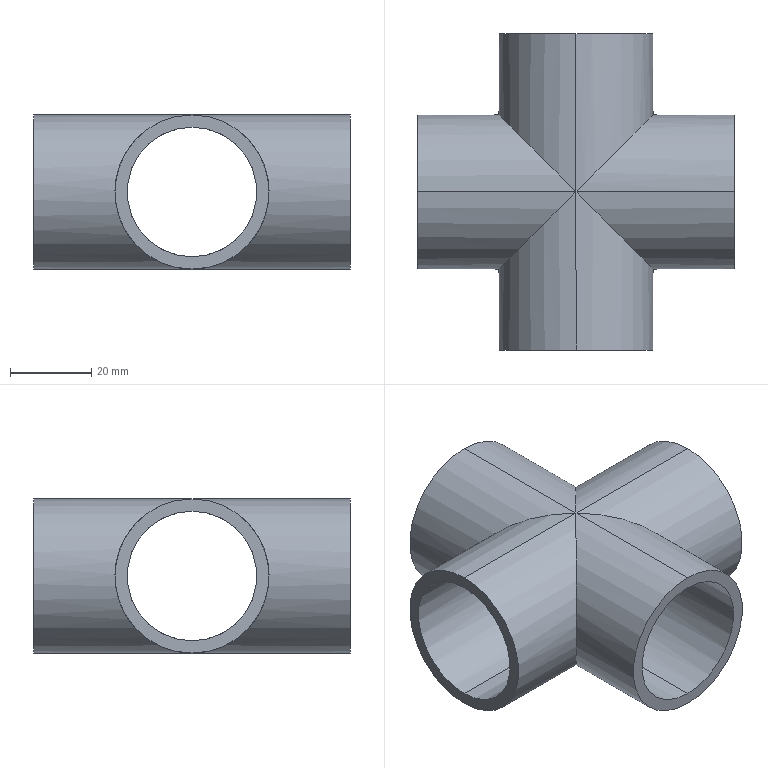Part | SolidWorks | features ICE 2, CirPattern 1, RefAxis 1, Revolution 1 | 1 solid | 20 faces | box 78 x 78 x 38 mm | volume 36723 mm3 | cylinder 16 | plane 4 | commonest cylinder face diameters 32 x8 38 x8
STEP:
#1=CARTESIAN_POINT('',(-39.,0.,16.));
#2=VERTEX_POINT('',#1);
#3=CARTESIAN_POINT('',(-39.,0.,-16.));
#4=VERTEX_POINT('',#3);
#5=CARTESIAN_POINT('',(-39.,0.,0.));
#6=DIRECTION('',(1.,0.,0.));
#7=DIRECTION('',(0.,0.,-1.));
#8=AXIS2_PLACEMENT_3D('',#5,#6,#7);
#9=CIRCLE('',#8,16.);
#10=EDGE_CURVE('',#2,#4,#9,.T.);
#11=ORIENTED_EDGE('',*,*,#10,.F.);
#12=CARTESIAN_POINT('',(0.,0.,16.));
#13=VERTEX_POINT('',#12);
#14=CARTESIAN_POINT('',(0.,0.,16.));
#15=DIRECTION('',(1.,0.,0.));
#16=VECTOR('',#15,1000.);
#17=LINE('',#14,#16);
#18=EDGE_CURVE('',#2,#13,#17,.T.);
#19=ORIENTED_EDGE('',*,*,#18,.T.);
#20=CARTESIAN_POINT('',(0.,0.,-16.));
#21=VERTEX_POINT('',#20);
#22=CARTESIAN_POINT('',(0.,0.,-16.));
#23=CARTESIAN_POINT('',(-32.,-32.,-16.));
#24=CARTESIAN_POINT('',(-32.,-32.,16.));
#25=CARTESIAN_POINT('',(0.,0.,16.));
#26=(BOUNDED_CURVE()B_SPLINE_CURVE(3,(#22,#23,#24,#25),.UNSPECIFIED.,.F.,.T.)B_SPLINE_CURVE_WITH_KNOTS((4,4),(4.712,7.854),.UNSPECIFIED.)CURVE()GEOMETRIC_REPRESENTATION_ITEM()RATIONAL_B_SPLINE_CURVE((1.,0.3333,0.3333,1.))REPRESENTATION_ITEM(''));
#27=EDGE_CURVE('',#21,#13,#26,.T.);
#28=ORIENTED_EDGE('',*,*,#27,.F.);
#29=CARTESIAN_POINT('',(0.,0.,-16.));
#30=DIRECTION('',(1.,0.,0.));
#31=VECTOR('',#30,1000.);
#32=LINE('',#29,#31);
#33=EDGE_CURVE('',#4,#21,#32,.T.);
#34=ORIENTED_EDGE('',*,*,#33,.F.);
#35=EDGE_LOOP('',(#11,#19,#28,#34));
#36=FACE_OUTER_BOUND('',#35,.T.);
#37=CARTESIAN_POINT('',(0.,0.,0.));
#38=DIRECTION('',(1.,0.,0.));
#39=DIRECTION('',(0.,0.,-1.));
#40=AXIS2_PLACEMENT_3D('',#37,#38,#39);
#41=CYLINDRICAL_SURFACE('',#40,16.);
#42=ADVANCED_FACE('',(#36),#41,.F.);
#43=CARTESIAN_POINT('',(0.,0.,16.));
#44=CARTESIAN_POINT('',(32.,-32.,16.));
#45=CARTESIAN_POINT('',(32.,-32.,-16.));
#46=CARTESIAN_POINT('',(0.,0.,-16.));
#47=(BOUNDED_CURVE()B_SPLINE_CURVE(3,(#43,#44,#45,#46),.UNSPECIFIED.,.F.,.F.)B_SPLINE_CURVE_WITH_KNOTS((4,4),(4.712,7.854),.UNSPECIFIED.)CURVE()GEOMETRIC_REPRESENTATION_ITEM()RATIONAL_B_SPLINE_CURVE((1.,0.3333,0.3333,1.))REPRESENTATION_ITEM(''));
#48=EDGE_CURVE('',#13,#21,#47,.T.);
#49=ORIENTED_EDGE('',*,*,#48,.F.);
#50=CARTESIAN_POINT('',(39.,0.,16.));
#51=VERTEX_POINT('',#50);
#52=CARTESIAN_POINT('',(0.,0.,16.));
#53=DIRECTION('',(1.,0.,0.));
#54=VECTOR('',#53,1000.);
#55=LINE('',#52,#54);
#56=EDGE_CURVE('',#13,#51,#55,.T.);
#57=ORIENTED_EDGE('',*,*,#56,.T.);
#58=CARTESIAN_POINT('',(39.,0.,-16.));
#59=VERTEX_POINT('',#58);
#60=CARTESIAN_POINT('',(39.,0.,0.));
#61=DIRECTION('',(-1.,0.,0.));
#62=DIRECTION('',(0.,0.,-1.));
#63=AXIS2_PLACEMENT_3D('',#60,#61,#62);
#64=CIRCLE('',#63,16.);
#65=EDGE_CURVE('',#59,#51,#64,.T.);
#66=ORIENTED_EDGE('',*,*,#65,.F.);
#67=CARTESIAN_POINT('',(0.,0.,-16.));
#68=DIRECTION('',(1.,0.,0.));
#69=VECTOR('',#68,1000.);
#70=LINE('',#67,#69);
#71=EDGE_CURVE('',#21,#59,#70,.T.);
#72=ORIENTED_EDGE('',*,*,#71,.F.);
#73=EDGE_LOOP('',(#49,#57,#66,#72));
#74=FACE_OUTER_BOUND('',#73,.T.);
#75=CARTESIAN_POINT('',(0.,0.,0.));
#76=DIRECTION('',(1.,0.,0.));
#77=DIRECTION('',(0.,0.,-1.));
#78=AXIS2_PLACEMENT_3D('',#75,#76,#77);
#79=CYLINDRICAL_SURFACE('',#78,16.);
#80=ADVANCED_FACE('',(#74),#79,.F.);
#81=CARTESIAN_POINT('',(0.,0.,-19.));
#82=VERTEX_POINT('',#81);
#83=CARTESIAN_POINT('',(0.,0.,19.));
#84=VERTEX_POINT('',#83);
#85=CARTESIAN_POINT('',(0.,0.,-19.));
#86=CARTESIAN_POINT('',(38.,38.,-19.));
#87=CARTESIAN_POINT('',(38.,38.,19.));
#88=CARTESIAN_POINT('',(0.,0.,19.));
#89=(BOUNDED_CURVE()B_SPLINE_CURVE(3,(#85,#86,#87,#88),.UNSPECIFIED.,.F.,.F.)B_SPLINE_CURVE_WITH_KNOTS((4,4),(1.571,4.712),.UNSPECIFIED.)CURVE()GEOMETRIC_REPRESENTATION_ITEM()RATIONAL_B_SPLINE_CURVE((1.,0.3333,0.3333,1.))REPRESENTATION_ITEM(''));
#90=EDGE_CURVE('',#82,#84,#89,.T.);
#91=ORIENTED_EDGE('',*,*,#90,.T.);
#92=CARTESIAN_POINT('',(39.,0.,19.));
#93=VERTEX_POINT('',#92);
#94=CARTESIAN_POINT('',(0.,0.,19.));
#95=DIRECTION('',(1.,0.,0.));
#96=VECTOR('',#95,1000.);
#97=LINE('',#94,#96);
#98=EDGE_CURVE('',#84,#93,#97,.T.);
#99=ORIENTED_EDGE('',*,*,#98,.T.);
#100=CARTESIAN_POINT('',(39.,0.,-19.));
#101=VERTEX_POINT('',#100);
#102=CARTESIAN_POINT('',(39.,0.,0.));
#103=DIRECTION('',(-1.,0.,0.));
#104=DIRECTION('',(0.,0.,-1.));
#105=AXIS2_PLACEMENT_3D('',#102,#103,#104);
#106=CIRCLE('',#105,19.);
#107=EDGE_CURVE('',#93,#101,#106,.T.);
#108=ORIENTED_EDGE('',*,*,#107,.T.);
#109=CARTESIAN_POINT('',(0.,0.,-19.));
#110=DIRECTION('',(1.,0.,0.));
#111=VECTOR('',#110,1000.);
#112=LINE('',#109,#111);
#113=EDGE_CURVE('',#82,#101,#112,.T.);
#114=ORIENTED_EDGE('',*,*,#113,.F.);
#115=EDGE_LOOP('',(#91,#99,#108,#114));
#116=FACE_OUTER_BOUND('',#115,.T.);
#117=CARTESIAN_POINT('',(0.,0.,0.));
#118=DIRECTION('',(1.,0.,0.));
#119=DIRECTION('',(0.,0.,-1.));
#120=AXIS2_PLACEMENT_3D('',#117,#118,#119);
#121=CYLINDRICAL_SURFACE('',#120,19.);
#122=ADVANCED_FACE('',(#116),#121,.T.);
#123=CARTESIAN_POINT('',(-39.,0.,-19.));
#124=VERTEX_POINT('',#123);
#125=CARTESIAN_POINT('',(-39.,0.,19.));
#126=VERTEX_POINT('',#125);
#127=CARTESIAN_POINT('',(-39.,0.,0.));
#128=DIRECTION('',(1.,0.,0.));
#129=DIRECTION('',(0.,0.,-1.));
#130=AXIS2_PLACEMENT_3D('',#127,#128,#129);
#131=CIRCLE('',#130,19.);
#132=EDGE_CURVE('',#124,#126,#131,.T.);
#133=ORIENTED_EDGE('',*,*,#132,.T.);
#134=CARTESIAN_POINT('',(0.,0.,19.));
#135=DIRECTION('',(1.,0.,0.));
#136=VECTOR('',#135,1000.);
#137=LINE('',#134,#136);
#138=EDGE_CURVE('',#126,#84,#137,.T.);
#139=ORIENTED_EDGE('',*,*,#138,.T.);
#140=CARTESIAN_POINT('',(0.,0.,19.));
#141=CARTESIAN_POINT('',(-38.,38.,19.));
#142=CARTESIAN_POINT('',(-38.,38.,-19.));
#143=CARTESIAN_POINT('',(0.,0.,-19.));
#144=(BOUNDED_CURVE()B_SPLINE_CURVE(3,(#140,#141,#142,#143),.UNSPECIFIED.,.F.,.F.)B_SPLINE_CURVE_WITH_KNOTS((4,4),(1.571,4.712),.UNSPECIFIED.)CURVE()GEOMETRIC_REPRESENTATION_ITEM()RATIONAL_B_SPLINE_CURVE((1.,0.3333,0.3333,1.))REPRESENTATION_ITEM(''));
#145=EDGE_CURVE('',#84,#82,#144,.T.);
#146=ORIENTED_EDGE('',*,*,#145,.T.);
#147=CARTESIAN_POINT('',(0.,0.,-19.));
#148=DIRECTION('',(1.,0.,0.));
#149=VECTOR('',#148,1000.);
#150=LINE('',#147,#149);
#151=EDGE_CURVE('',#124,#82,#150,.T.);
#152=ORIENTED_EDGE('',*,*,#151,.F.);
#153=EDGE_LOOP('',(#133,#139,#146,#152));
#154=FACE_OUTER_BOUND('',#153,.T.);
#155=CARTESIAN_POINT('',(0.,0.,0.));
#156=DIRECTION('',(1.,0.,0.));
#157=DIRECTION('',(0.,0.,-1.));
#158=AXIS2_PLACEMENT_3D('',#155,#156,#157);
#159=CYLINDRICAL_SURFACE('',#158,19.);
#160=ADVANCED_FACE('',(#154),#159,.T.);
#161=CARTESIAN_POINT('',(0.,-39.,-19.));
#162=VERTEX_POINT('',#161);
#163=CARTESIAN_POINT('',(0.,-39.,19.));
#164=VERTEX_POINT('',#163);
#165=CARTESIAN_POINT('',(0.,-39.,0.));
#166=DIRECTION('',(0.,1.,0.));
#167=DIRECTION('',(0.,0.,-1.));
#168=AXIS2_PLACEMENT_3D('',#165,#166,#167);
#169=CIRCLE('',#168,19.);
#170=EDGE_CURVE('',#162,#164,#169,.T.);
#171=ORIENTED_EDGE('',*,*,#170,.T.);
#172=CARTESIAN_POINT('',(0.,0.,19.));
#173=DIRECTION('',(0.,1.,0.));
#174=VECTOR('',#173,1000.);
#175=LINE('',#172,#174);
#176=EDGE_CURVE('',#164,#84,#175,.T.);
#177=ORIENTED_EDGE('',*,*,#176,.T.);
#178=CARTESIAN_POINT('',(0.,0.,19.));
#179=CARTESIAN_POINT('',(-38.,-38.,19.));
#180=CARTESIAN_POINT('',(-38.,-38.,-19.));
#181=CARTESIAN_POINT('',(0.,0.,-19.));
#182=(BOUNDED_CURVE()B_SPLINE_CURVE(3,(#178,#179,#180,#181),.UNSPECIFIED.,.F.,.F.)B_SPLINE_CURVE_WITH_KNOTS((4,4),(1.571,4.712),.UNSPECIFIED.)CURVE()GEOMETRIC_REPRESENTATION_ITEM()RATIONAL_B_SPLINE_CURVE((1.,0.3333,0.3333,1.))REPRESENTATION_ITEM(''));
#183=EDGE_CURVE('',#84,#82,#182,.T.);
#184=ORIENTED_EDGE('',*,*,#183,.T.);
#185=CARTESIAN_POINT('',(0.,0.,-19.));
#186=DIRECTION('',(0.,1.,0.));
#187=VECTOR('',#186,1000.);
#188=LINE('',#185,#187);
#189=EDGE_CURVE('',#162,#82,#188,.T.);
#190=ORIENTED_EDGE('',*,*,#189,.F.);
#191=EDGE_LOOP('',(#171,#177,#184,#190));
#192=FACE_OUTER_BOUND('',#191,.T.);
#193=CARTESIAN_POINT('',(0.,0.,0.));
#194=DIRECTION('',(0.,1.,0.));
#195=DIRECTION('',(0.,0.,-1.));
#196=AXIS2_PLACEMENT_3D('',#193,#194,#195);
#197=CYLINDRICAL_SURFACE('',#196,19.);
#198=ADVANCED_FACE('',(#192),#197,.T.);
#199=CARTESIAN_POINT('',(0.,39.,-19.));
#200=VERTEX_POINT('',#199);
#201=CARTESIAN_POINT('',(0.,39.,19.));
#202=VERTEX_POINT('',#201);
#203=CARTESIAN_POINT('',(0.,39.,0.));
#204=DIRECTION('',(0.,-1.,0.));
#205=DIRECTION('',(0.,0.,-1.));
#206=AXIS2_PLACEMENT_3D('',#203,#204,#205);
#207=CIRCLE('',#206,19.);
#208=EDGE_CURVE('',#200,#202,#207,.T.);
#209=ORIENTED_EDGE('',*,*,#208,.T.);
#210=CARTESIAN_POINT('',(0.,0.,19.));
#211=DIRECTION('',(0.,-1.,0.));
#212=VECTOR('',#211,1000.);
#213=LINE('',#210,#212);
#214=EDGE_CURVE('',#202,#84,#213,.T.);
#215=ORIENTED_EDGE('',*,*,#214,.T.);
#216=ORIENTED_EDGE('',*,*,#90,.F.);
#217=CARTESIAN_POINT('',(0.,0.,-19.));
#218=DIRECTION('',(0.,-1.,0.));
#219=VECTOR('',#218,1000.);
#220=LINE('',#217,#219);
#221=EDGE_CURVE('',#200,#82,#220,.T.);
#222=ORIENTED_EDGE('',*,*,#221,.F.);
#223=EDGE_LOOP('',(#209,#215,#216,#222));
#224=FACE_OUTER_BOUND('',#223,.T.);
#225=CARTESIAN_POINT('',(0.,0.,0.));
#226=DIRECTION('',(0.,-1.,0.));
#227=DIRECTION('',(0.,0.,-1.));
#228=AXIS2_PLACEMENT_3D('',#225,#226,#227);
#229=CYLINDRICAL_SURFACE('',#228,19.);
#230=ADVANCED_FACE('',(#224),#229,.T.);
#231=CARTESIAN_POINT('',(0.,39.,16.));
#232=VERTEX_POINT('',#231);
#233=CARTESIAN_POINT('',(0.,39.,-16.));
#234=VERTEX_POINT('',#233);
#235=CARTESIAN_POINT('',(0.,39.,0.));
#236=DIRECTION('',(0.,-1.,0.));
#237=DIRECTION('',(0.,0.,-1.));
#238=AXIS2_PLACEMENT_3D('',#235,#236,#237);
#239=CIRCLE('',#238,16.);
#240=EDGE_CURVE('',#232,#234,#239,.T.);
#241=ORIENTED_EDGE('',*,*,#240,.F.);
#242=CARTESIAN_POINT('',(0.,0.,16.));
#243=DIRECTION('',(0.,-1.,0.));
#244=VECTOR('',#243,1000.);
#245=LINE('',#242,#244);
#246=EDGE_CURVE('',#232,#13,#245,.T.);
#247=ORIENTED_EDGE('',*,*,#246,.T.);
#248=CARTESIAN_POINT('',(0.,0.,16.));
#249=CARTESIAN_POINT('',(-32.,32.,16.));
#250=CARTESIAN_POINT('',(-32.,32.,-16.));
#251=CARTESIAN_POINT('',(0.,0.,-16.));
#252=(BOUNDED_CURVE()B_SPLINE_CURVE(3,(#248,#249,#250,#251),.UNSPECIFIED.,.F.,.F.)B_SPLINE_CURVE_WITH_KNOTS((4,4),(1.571,4.712),.UNSPECIFIED.)CURVE()GEOMETRIC_REPRESENTATION_ITEM()RATIONAL_B_SPLINE_CURVE((1.,0.3333,0.3333,1.))REPRESENTATION_ITEM(''));
#253=EDGE_CURVE('',#13,#21,#252,.T.);
#254=ORIENTED_EDGE('',*,*,#253,.T.);
#255=CARTESIAN_POINT('',(0.,0.,-16.));
#256=DIRECTION('',(0.,-1.,0.));
#257=VECTOR('',#256,1000.);
#258=LINE('',#255,#257);
#259=EDGE_CURVE('',#234,#21,#258,.T.);
#260=ORIENTED_EDGE('',*,*,#259,.F.);
#261=EDGE_LOOP('',(#241,#247,#254,#260));
#262=FACE_OUTER_BOUND('',#261,.T.);
#263=CARTESIAN_POINT('',(0.,0.,0.));
#264=DIRECTION('',(0.,-1.,0.));
#265=DIRECTION('',(0.,0.,-1.));
#266=AXIS2_PLACEMENT_3D('',#263,#264,#265);
#267=CYLINDRICAL_SURFACE('',#266,16.);
#268=ADVANCED_FACE('',(#262),#267,.F.);
#269=ORIENTED_EDGE('',*,*,#27,.T.);
#270=CARTESIAN_POINT('',(0.,-39.,16.));
#271=VERTEX_POINT('',#270);
#272=CARTESIAN_POINT('',(0.,0.,16.));
#273=DIRECTION('',(0.,-1.,0.));
#274=VECTOR('',#273,1000.);
#275=LINE('',#272,#274);
#276=EDGE_CURVE('',#13,#271,#275,.T.);
#277=ORIENTED_EDGE('',*,*,#276,.T.);
#278=CARTESIAN_POINT('',(0.,-39.,-16.));
#279=VERTEX_POINT('',#278);
#280=CARTESIAN_POINT('',(0.,-39.,0.));
#281=DIRECTION('',(0.,1.,0.));
#282=DIRECTION('',(0.,0.,-1.));
#283=AXIS2_PLACEMENT_3D('',#280,#281,#282);
#284=CIRCLE('',#283,16.);
#285=EDGE_CURVE('',#279,#271,#284,.T.);
#286=ORIENTED_EDGE('',*,*,#285,.F.);
#287=CARTESIAN_POINT('',(0.,0.,-16.));
#288=DIRECTION('',(0.,-1.,0.));
#289=VECTOR('',#288,1000.);
#290=LINE('',#287,#289);
#291=EDGE_CURVE('',#21,#279,#290,.T.);
#292=ORIENTED_EDGE('',*,*,#291,.F.);
#293=EDGE_LOOP('',(#269,#277,#286,#292));
#294=FACE_OUTER_BOUND('',#293,.T.);
#295=CARTESIAN_POINT('',(0.,0.,0.));
#296=DIRECTION('',(0.,-1.,0.));
#297=DIRECTION('',(0.,0.,-1.));
#298=AXIS2_PLACEMENT_3D('',#295,#296,#297);
#299=CYLINDRICAL_SURFACE('',#298,16.);
#300=ADVANCED_FACE('',(#294),#299,.F.);
#301=ORIENTED_EDGE('',*,*,#276,.F.);
#302=ORIENTED_EDGE('',*,*,#48,.T.);
#303=ORIENTED_EDGE('',*,*,#291,.T.);
#304=CARTESIAN_POINT('',(0.,-39.,0.));
#305=DIRECTION('',(0.,1.,0.));
#306=DIRECTION('',(0.,0.,-1.));
#307=AXIS2_PLACEMENT_3D('',#304,#305,#306);
#308=CIRCLE('',#307,16.);
#309=EDGE_CURVE('',#271,#279,#308,.T.);
#310=ORIENTED_EDGE('',*,*,#309,.F.);
#311=EDGE_LOOP('',(#301,#302,#303,#310));
#312=FACE_OUTER_BOUND('',#311,.T.);
#313=CARTESIAN_POINT('',(0.,0.,0.));
#314=DIRECTION('',(0.,-1.,0.));
#315=DIRECTION('',(0.,0.,-1.));
#316=AXIS2_PLACEMENT_3D('',#313,#314,#315);
#317=CYLINDRICAL_SURFACE('',#316,16.);
#318=ADVANCED_FACE('',(#312),#317,.F.);
#319=ORIENTED_EDGE('',*,*,#246,.F.);
#320=CARTESIAN_POINT('',(0.,39.,0.));
#321=DIRECTION('',(0.,-1.,0.));
#322=DIRECTION('',(0.,0.,-1.));
#323=AXIS2_PLACEMENT_3D('',#320,#321,#322);
#324=CIRCLE('',#323,16.);
#325=EDGE_CURVE('',#234,#232,#324,.T.);
#326=ORIENTED_EDGE('',*,*,#325,.F.);
#327=ORIENTED_EDGE('',*,*,#259,.T.);
#328=CARTESIAN_POINT('',(0.,0.,-16.));
#329=CARTESIAN_POINT('',(32.,32.,-16.));
#330=CARTESIAN_POINT('',(32.,32.,16.));
#331=CARTESIAN_POINT('',(0.,0.,16.));
#332=(BOUNDED_CURVE()B_SPLINE_CURVE(3,(#328,#329,#330,#331),.UNSPECIFIED.,.F.,.F.)B_SPLINE_CURVE_WITH_KNOTS((4,4),(1.571,4.712),.UNSPECIFIED.)CURVE()GEOMETRIC_REPRESENTATION_ITEM()RATIONAL_B_SPLINE_CURVE((1.,0.3333,0.3333,1.))REPRESENTATION_ITEM(''));
#333=EDGE_CURVE('',#21,#13,#332,.T.);
#334=ORIENTED_EDGE('',*,*,#333,.T.);
#335=EDGE_LOOP('',(#319,#326,#327,#334));
#336=FACE_OUTER_BOUND('',#335,.T.);
#337=CARTESIAN_POINT('',(0.,0.,0.));
#338=DIRECTION('',(0.,-1.,0.));
#339=DIRECTION('',(0.,0.,-1.));
#340=AXIS2_PLACEMENT_3D('',#337,#338,#339);
#341=CYLINDRICAL_SURFACE('',#340,16.);
#342=ADVANCED_FACE('',(#336),#341,.F.);
#343=ORIENTED_EDGE('',*,*,#214,.F.);
#344=CARTESIAN_POINT('',(0.,39.,0.));
#345=DIRECTION('',(0.,-1.,0.));
#346=DIRECTION('',(0.,0.,-1.));
#347=AXIS2_PLACEMENT_3D('',#344,#345,#346);
#348=CIRCLE('',#347,19.);
#349=EDGE_CURVE('',#202,#200,#348,.T.);
#350=ORIENTED_EDGE('',*,*,#349,.T.);
#351=ORIENTED_EDGE('',*,*,#221,.T.);
#352=ORIENTED_EDGE('',*,*,#145,.F.);
#353=EDGE_LOOP('',(#343,#350,#351,#352));
#354=FACE_OUTER_BOUND('',#353,.T.);
#355=CARTESIAN_POINT('',(0.,0.,0.));
#356=DIRECTION('',(0.,-1.,0.));
#357=DIRECTION('',(0.,0.,-1.));
#358=AXIS2_PLACEMENT_3D('',#355,#356,#357);
#359=CYLINDRICAL_SURFACE('',#358,19.);
#360=ADVANCED_FACE('',(#354),#359,.T.);
#361=ORIENTED_EDGE('',*,*,#208,.F.);
#362=ORIENTED_EDGE('',*,*,#349,.F.);
#363=EDGE_LOOP('',(#361,#362));
#364=FACE_OUTER_BOUND('',#363,.T.);
#365=ORIENTED_EDGE('',*,*,#325,.T.);
#366=ORIENTED_EDGE('',*,*,#240,.T.);
#367=EDGE_LOOP('',(#365,#366));
#368=FACE_BOUND('',#367,.T.);
#369=CARTESIAN_POINT('',(-16.,39.,0.));
#370=DIRECTION('',(0.,-1.,0.));
#371=DIRECTION('',(0.,0.,-1.));
#372=AXIS2_PLACEMENT_3D('',#369,#370,#371);
#373=PLANE('',#372);
#374=ADVANCED_FACE('',(#364,#368),#373,.F.);
#375=ORIENTED_EDGE('',*,*,#176,.F.);
#376=CARTESIAN_POINT('',(0.,-39.,0.));
#377=DIRECTION('',(0.,1.,0.));
#378=DIRECTION('',(0.,0.,-1.));
#379=AXIS2_PLACEMENT_3D('',#376,#377,#378);
#380=CIRCLE('',#379,19.);
#381=EDGE_CURVE('',#164,#162,#380,.T.);
#382=ORIENTED_EDGE('',*,*,#381,.T.);
#383=ORIENTED_EDGE('',*,*,#189,.T.);
#384=CARTESIAN_POINT('',(0.,0.,19.));
#385=CARTESIAN_POINT('',(38.,-38.,19.));
#386=CARTESIAN_POINT('',(38.,-38.,-19.));
#387=CARTESIAN_POINT('',(0.,0.,-19.));
#388=(BOUNDED_CURVE()B_SPLINE_CURVE(3,(#384,#385,#386,#387),.UNSPECIFIED.,.F.,.F.)B_SPLINE_CURVE_WITH_KNOTS((4,4),(1.571,4.712),.UNSPECIFIED.)CURVE()GEOMETRIC_REPRESENTATION_ITEM()RATIONAL_B_SPLINE_CURVE((1.,0.3333,0.3333,1.))REPRESENTATION_ITEM(''));
#389=EDGE_CURVE('',#84,#82,#388,.T.);
#390=ORIENTED_EDGE('',*,*,#389,.F.);
#391=EDGE_LOOP('',(#375,#382,#383,#390));
#392=FACE_OUTER_BOUND('',#391,.T.);
#393=CARTESIAN_POINT('',(0.,0.,0.));
#394=DIRECTION('',(0.,1.,0.));
#395=DIRECTION('',(0.,0.,-1.));
#396=AXIS2_PLACEMENT_3D('',#393,#394,#395);
#397=CYLINDRICAL_SURFACE('',#396,19.);
#398=ADVANCED_FACE('',(#392),#397,.T.);
#399=ORIENTED_EDGE('',*,*,#170,.F.);
#400=ORIENTED_EDGE('',*,*,#381,.F.);
#401=EDGE_LOOP('',(#399,#400));
#402=FACE_OUTER_BOUND('',#401,.T.);
#403=ORIENTED_EDGE('',*,*,#285,.T.);
#404=ORIENTED_EDGE('',*,*,#309,.T.);
#405=EDGE_LOOP('',(#403,#404));
#406=FACE_BOUND('',#405,.T.);
#407=CARTESIAN_POINT('',(16.,-39.,0.));
#408=DIRECTION('',(0.,1.,0.));
#409=DIRECTION('',(0.,0.,-1.));
#410=AXIS2_PLACEMENT_3D('',#407,#408,#409);
#411=PLANE('',#410);
#412=ADVANCED_FACE('',(#402,#406),#411,.F.);
#413=CARTESIAN_POINT('',(39.,0.,0.));
#414=DIRECTION('',(-1.,0.,0.));
#415=DIRECTION('',(0.,0.,-1.));
#416=AXIS2_PLACEMENT_3D('',#413,#414,#415);
#417=CIRCLE('',#416,19.);
#418=EDGE_CURVE('',#101,#93,#417,.T.);
#419=ORIENTED_EDGE('',*,*,#418,.F.);
#420=ORIENTED_EDGE('',*,*,#107,.F.);
#421=EDGE_LOOP('',(#419,#420));
#422=FACE_OUTER_BOUND('',#421,.T.);
#423=ORIENTED_EDGE('',*,*,#65,.T.);
#424=CARTESIAN_POINT('',(39.,0.,0.));
#425=DIRECTION('',(-1.,0.,0.));
#426=DIRECTION('',(0.,0.,-1.));
#427=AXIS2_PLACEMENT_3D('',#424,#425,#426);
#428=CIRCLE('',#427,16.);
#429=EDGE_CURVE('',#51,#59,#428,.T.);
#430=ORIENTED_EDGE('',*,*,#429,.T.);
#431=EDGE_LOOP('',(#423,#430));
#432=FACE_BOUND('',#431,.T.);
#433=CARTESIAN_POINT('',(39.,16.,0.));
#434=DIRECTION('',(-1.,0.,0.));
#435=DIRECTION('',(0.,0.,-1.));
#436=AXIS2_PLACEMENT_3D('',#433,#434,#435);
#437=PLANE('',#436);
#438=ADVANCED_FACE('',(#422,#432),#437,.F.);
#439=ORIENTED_EDGE('',*,*,#132,.F.);
#440=CARTESIAN_POINT('',(-39.,0.,0.));
#441=DIRECTION('',(1.,0.,0.));
#442=DIRECTION('',(0.,0.,-1.));
#443=AXIS2_PLACEMENT_3D('',#440,#441,#442);
#444=CIRCLE('',#443,19.);
#445=EDGE_CURVE('',#126,#124,#444,.T.);
#446=ORIENTED_EDGE('',*,*,#445,.F.);
#447=EDGE_LOOP('',(#439,#446));
#448=FACE_OUTER_BOUND('',#447,.T.);
#449=CARTESIAN_POINT('',(-39.,0.,0.));
#450=DIRECTION('',(1.,0.,0.));
#451=DIRECTION('',(0.,0.,-1.));
#452=AXIS2_PLACEMENT_3D('',#449,#450,#451);
#453=CIRCLE('',#452,16.);
#454=EDGE_CURVE('',#4,#2,#453,.T.);
#455=ORIENTED_EDGE('',*,*,#454,.T.);
#456=ORIENTED_EDGE('',*,*,#10,.T.);
#457=EDGE_LOOP('',(#455,#456));
#458=FACE_BOUND('',#457,.T.);
#459=CARTESIAN_POINT('',(-39.,-16.,0.));
#460=DIRECTION('',(1.,0.,0.));
#461=DIRECTION('',(0.,0.,-1.));
#462=AXIS2_PLACEMENT_3D('',#459,#460,#461);
#463=PLANE('',#462);
#464=ADVANCED_FACE('',(#448,#458),#463,.F.);
#465=ORIENTED_EDGE('',*,*,#138,.F.);
#466=ORIENTED_EDGE('',*,*,#445,.T.);
#467=ORIENTED_EDGE('',*,*,#151,.T.);
#468=ORIENTED_EDGE('',*,*,#183,.F.);
#469=EDGE_LOOP('',(#465,#466,#467,#468));
#470=FACE_OUTER_BOUND('',#469,.T.);
#471=CARTESIAN_POINT('',(0.,0.,0.));
#472=DIRECTION('',(1.,0.,0.));
#473=DIRECTION('',(0.,0.,-1.));
#474=AXIS2_PLACEMENT_3D('',#471,#472,#473);
#475=CYLINDRICAL_SURFACE('',#474,19.);
#476=ADVANCED_FACE('',(#470),#475,.T.);
#477=ORIENTED_EDGE('',*,*,#98,.F.);
#478=ORIENTED_EDGE('',*,*,#389,.T.);
#479=ORIENTED_EDGE('',*,*,#113,.T.);
#480=ORIENTED_EDGE('',*,*,#418,.T.);
#481=EDGE_LOOP('',(#477,#478,#479,#480));
#482=FACE_OUTER_BOUND('',#481,.T.);
#483=CARTESIAN_POINT('',(0.,0.,0.));
#484=DIRECTION('',(1.,0.,0.));
#485=DIRECTION('',(0.,0.,-1.));
#486=AXIS2_PLACEMENT_3D('',#483,#484,#485);
#487=CYLINDRICAL_SURFACE('',#486,19.);
#488=ADVANCED_FACE('',(#482),#487,.T.);
#489=ORIENTED_EDGE('',*,*,#56,.F.);
#490=ORIENTED_EDGE('',*,*,#333,.F.);
#491=ORIENTED_EDGE('',*,*,#71,.T.);
#492=ORIENTED_EDGE('',*,*,#429,.F.);
#493=EDGE_LOOP('',(#489,#490,#491,#492));
#494=FACE_OUTER_BOUND('',#493,.T.);
#495=CARTESIAN_POINT('',(0.,0.,0.));
#496=DIRECTION('',(1.,0.,0.));
#497=DIRECTION('',(0.,0.,-1.));
#498=AXIS2_PLACEMENT_3D('',#495,#496,#497);
#499=CYLINDRICAL_SURFACE('',#498,16.);
#500=ADVANCED_FACE('',(#494),#499,.F.);
#501=ORIENTED_EDGE('',*,*,#18,.F.);
#502=ORIENTED_EDGE('',*,*,#454,.F.);
#503=ORIENTED_EDGE('',*,*,#33,.T.);
#504=ORIENTED_EDGE('',*,*,#253,.F.);
#505=EDGE_LOOP('',(#501,#502,#503,#504));
#506=FACE_OUTER_BOUND('',#505,.T.);
#507=CARTESIAN_POINT('',(0.,0.,0.));
#508=DIRECTION('',(1.,0.,0.));
#509=DIRECTION('',(0.,0.,-1.));
#510=AXIS2_PLACEMENT_3D('',#507,#508,#509);
#511=CYLINDRICAL_SURFACE('',#510,16.);
#512=ADVANCED_FACE('',(#506),#511,.F.);
#513=CLOSED_SHELL('',(#42,#80,#122,#160,#198,#230,#268,#300,#318,#342,#360,#374,#398,#412,#438,#464,#476,#488,#500,#512));
#514=MANIFOLD_SOLID_BREP('',#513);
#515=CARTESIAN_POINT('',(0.,0.,0.));
#516=DIRECTION('',(0.,0.,1.));
#517=DIRECTION('',(1.,0.,0.));
#518=AXIS2_PLACEMENT_3D('',#515,#516,#517);
#519=(LENGTH_UNIT()NAMED_UNIT(*)SI_UNIT(.MILLI.,.METRE.));
#520=UNCERTAINTY_MEASURE_WITH_UNIT(LENGTH_MEASURE(0.00001),#519,'','');
#521=(NAMED_UNIT(*)PLANE_ANGLE_UNIT()SI_UNIT($,.RADIAN.));
#522=(NAMED_UNIT(*)SI_UNIT($,.STERADIAN.)SOLID_ANGLE_UNIT());
#523=(GEOMETRIC_REPRESENTATION_CONTEXT(3)GLOBAL_UNCERTAINTY_ASSIGNED_CONTEXT((#520))GLOBAL_UNIT_ASSIGNED_CONTEXT((#519,#521,#522))REPRESENTATION_CONTEXT('',''));
#524=ADVANCED_BREP_SHAPE_REPRESENTATION('',(#514,#518),#523);